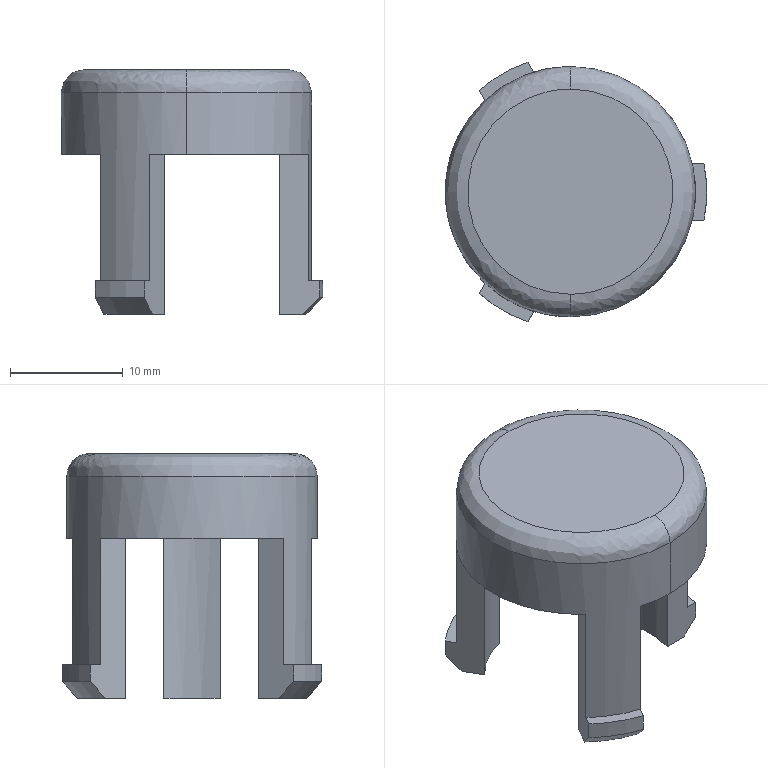Part | SolidWorks | features BaseBody 1 | 1 solid | 30 faces | box 23.2 x 23.006 x 21.7 mm | volume 2251 mm3 | plane 17 | cylinder 7 | cone 4 | spline 2 | commonest cylinder face diameters 24.2 x3 17.2 x2 22.2 x2
STEP:
#1=CARTESIAN_POINT('',(35.731,-11.1,14.8));
#2=VERTEX_POINT('',#1);
#3=CARTESIAN_POINT('',(35.731,11.1,14.8));
#4=VERTEX_POINT('',#3);
#5=CARTESIAN_POINT('',(35.731,0.,14.8));
#6=DIRECTION('',(0.,0.,-1.));
#7=DIRECTION('',(0.,1.,0.));
#8=AXIS2_PLACEMENT_3D('',#5,#6,#7);
#9=CIRCLE('',#8,11.1);
#10=EDGE_CURVE('',#2,#4,#9,.T.);
#11=ORIENTED_EDGE('',*,*,#10,.F.);
#12=CARTESIAN_POINT('',(35.731,-9.1,16.8));
#13=VERTEX_POINT('',#12);
#14=CARTESIAN_POINT('',(35.731,-9.1,14.8));
#15=DIRECTION('',(-1.,0.,0.));
#16=DIRECTION('',(0.,-1.,0.));
#17=AXIS2_PLACEMENT_3D('',#14,#15,#16);
#18=CIRCLE('',#17,2.);
#19=EDGE_CURVE('',#2,#13,#18,.T.);
#20=ORIENTED_EDGE('',*,*,#19,.T.);
#21=CARTESIAN_POINT('',(35.731,9.1,16.8));
#22=VERTEX_POINT('',#21);
#23=CARTESIAN_POINT('',(35.731,-9.1,16.8));
#24=CARTESIAN_POINT('',(17.531,-9.1,16.8));
#25=CARTESIAN_POINT('',(17.531,9.1,16.8));
#26=CARTESIAN_POINT('',(35.731,9.1,16.8));
#27=(BOUNDED_CURVE()B_SPLINE_CURVE(3,(#23,#24,#25,#26),.UNSPECIFIED.,.F.,.T.)B_SPLINE_CURVE_WITH_KNOTS((4,4),(0.,1.),.UNSPECIFIED.)CURVE()GEOMETRIC_REPRESENTATION_ITEM()RATIONAL_B_SPLINE_CURVE((1.,0.3333,0.3333,1.))REPRESENTATION_ITEM(''));
#28=EDGE_CURVE('',#13,#22,#27,.T.);
#29=ORIENTED_EDGE('',*,*,#28,.T.);
#30=CARTESIAN_POINT('',(35.731,9.1,14.8));
#31=DIRECTION('',(1.,0.,0.));
#32=DIRECTION('',(0.,1.,0.));
#33=AXIS2_PLACEMENT_3D('',#30,#31,#32);
#34=CIRCLE('',#33,2.);
#35=EDGE_CURVE('',#4,#22,#34,.T.);
#36=ORIENTED_EDGE('',*,*,#35,.F.);
#37=EDGE_LOOP('',(#11,#20,#29,#36));
#38=FACE_OUTER_BOUND('',#37,.T.);
#39=CARTESIAN_POINT('',(35.731,-11.1,14.8));
#40=CARTESIAN_POINT('',(13.531,-11.1,14.8));
#41=CARTESIAN_POINT('',(13.531,11.1,14.8));
#42=CARTESIAN_POINT('',(35.731,11.1,14.8));
#43=CARTESIAN_POINT('',(35.731,-11.1,15.972));
#44=CARTESIAN_POINT('',(13.531,-11.1,15.972));
#45=CARTESIAN_POINT('',(13.531,11.1,15.972));
#46=CARTESIAN_POINT('',(35.731,11.1,15.972));
#47=CARTESIAN_POINT('',(35.731,-10.272,16.8));
#48=CARTESIAN_POINT('',(15.187,-10.272,16.8));
#49=CARTESIAN_POINT('',(15.187,10.272,16.8));
#50=CARTESIAN_POINT('',(35.731,10.272,16.8));
#51=CARTESIAN_POINT('',(35.731,-9.1,16.8));
#52=CARTESIAN_POINT('',(17.531,-9.1,16.8));
#53=CARTESIAN_POINT('',(17.531,9.1,16.8));
#54=CARTESIAN_POINT('',(35.731,9.1,16.8));
#55=(BOUNDED_SURFACE()B_SPLINE_SURFACE(3,3,((#39,#40,#41,#42),(#43,#44,#45,#46),(#47,#48,#49,#50),(#51,#52,#53,#54)),.UNSPECIFIED.,.F.,.F.,.F.)B_SPLINE_SURFACE_WITH_KNOTS((4,4),(4,4),(0.,1.),(0.,1.),.UNSPECIFIED.)GEOMETRIC_REPRESENTATION_ITEM()RATIONAL_B_SPLINE_SURFACE(((1.,0.3333,0.3333,1.),(0.8047,0.2682,0.2682,0.8047),(0.8047,0.2682,0.2682,0.8047),(1.,0.3333,0.3333,1.)))REPRESENTATION_ITEM('')SURFACE());
#56=ADVANCED_FACE('',(#38),#55,.T.);
#57=CARTESIAN_POINT('',(35.731,0.,14.8));
#58=DIRECTION('',(0.,0.,-1.));
#59=DIRECTION('',(0.,1.,0.));
#60=AXIS2_PLACEMENT_3D('',#57,#58,#59);
#61=CIRCLE('',#60,11.1);
#62=EDGE_CURVE('',#4,#2,#61,.T.);
#63=ORIENTED_EDGE('',*,*,#62,.T.);
#64=CARTESIAN_POINT('',(35.731,-11.1,9.3));
#65=VERTEX_POINT('',#64);
#66=CARTESIAN_POINT('',(35.731,-11.1,53.496));
#67=DIRECTION('',(0.,0.,-1.));
#68=VECTOR('',#67,1000.);
#69=LINE('',#66,#68);
#70=EDGE_CURVE('',#2,#65,#69,.T.);
#71=ORIENTED_EDGE('',*,*,#70,.T.);
#72=CARTESIAN_POINT('',(46.545,-2.5,9.3));
#73=VERTEX_POINT('',#72);
#74=CARTESIAN_POINT('',(35.731,0.,9.3));
#75=DIRECTION('',(0.,0.,1.));
#76=DIRECTION('',(0.,1.,0.));
#77=AXIS2_PLACEMENT_3D('',#74,#75,#76);
#78=CIRCLE('',#77,11.1);
#79=EDGE_CURVE('',#65,#73,#78,.T.);
#80=ORIENTED_EDGE('',*,*,#79,.T.);
#81=CARTESIAN_POINT('',(46.545,-2.5,-1.9));
#82=VERTEX_POINT('',#81);
#83=CARTESIAN_POINT('',(46.545,-2.5,53.496));
#84=DIRECTION('',(0.,0.,-1.));
#85=VECTOR('',#84,1000.);
#86=LINE('',#83,#85);
#87=EDGE_CURVE('',#73,#82,#86,.T.);
#88=ORIENTED_EDGE('',*,*,#87,.T.);
#89=CARTESIAN_POINT('',(46.545,2.5,-1.9));
#90=VERTEX_POINT('',#89);
#91=CARTESIAN_POINT('',(35.731,0.,-1.9));
#92=DIRECTION('',(0.,0.,1.));
#93=DIRECTION('',(0.,1.,0.));
#94=AXIS2_PLACEMENT_3D('',#91,#92,#93);
#95=CIRCLE('',#94,11.1);
#96=EDGE_CURVE('',#82,#90,#95,.T.);
#97=ORIENTED_EDGE('',*,*,#96,.T.);
#98=CARTESIAN_POINT('',(46.545,2.5,9.3));
#99=VERTEX_POINT('',#98);
#100=CARTESIAN_POINT('',(46.545,2.5,53.496));
#101=DIRECTION('',(0.,0.,1.));
#102=VECTOR('',#101,1000.);
#103=LINE('',#100,#102);
#104=EDGE_CURVE('',#90,#99,#103,.T.);
#105=ORIENTED_EDGE('',*,*,#104,.T.);
#106=CARTESIAN_POINT('',(35.731,11.1,9.3));
#107=VERTEX_POINT('',#106);
#108=CARTESIAN_POINT('',(35.731,0.,9.3));
#109=DIRECTION('',(0.,0.,1.));
#110=DIRECTION('',(0.,1.,0.));
#111=AXIS2_PLACEMENT_3D('',#108,#109,#110);
#112=CIRCLE('',#111,11.1);
#113=EDGE_CURVE('',#99,#107,#112,.T.);
#114=ORIENTED_EDGE('',*,*,#113,.T.);
#115=CARTESIAN_POINT('',(35.731,11.1,53.496));
#116=DIRECTION('',(0.,0.,-1.));
#117=VECTOR('',#116,1000.);
#118=LINE('',#115,#117);
#119=EDGE_CURVE('',#4,#107,#118,.T.);
#120=ORIENTED_EDGE('',*,*,#119,.F.);
#121=EDGE_LOOP('',(#63,#71,#80,#88,#97,#105,#114,#120));
#122=FACE_OUTER_BOUND('',#121,.T.);
#123=CARTESIAN_POINT('',(35.731,0.,53.496));
#124=DIRECTION('',(0.,0.,-1.));
#125=DIRECTION('',(0.,1.,0.));
#126=AXIS2_PLACEMENT_3D('',#123,#124,#125);
#127=CYLINDRICAL_SURFACE('',#126,11.1);
#128=ADVANCED_FACE('',(#122),#127,.T.);
#129=CARTESIAN_POINT('',(35.731,-8.6,14.3));
#130=VERTEX_POINT('',#129);
#131=CARTESIAN_POINT('',(35.731,8.6,14.3));
#132=VERTEX_POINT('',#131);
#133=CARTESIAN_POINT('',(35.731,0.,14.3));
#134=DIRECTION('',(0.,0.,-1.));
#135=DIRECTION('',(0.,1.,0.));
#136=AXIS2_PLACEMENT_3D('',#133,#134,#135);
#137=CIRCLE('',#136,8.6);
#138=EDGE_CURVE('',#130,#132,#137,.T.);
#139=ORIENTED_EDGE('',*,*,#138,.F.);
#140=CARTESIAN_POINT('',(35.731,-8.6,9.3));
#141=VERTEX_POINT('',#140);
#142=CARTESIAN_POINT('',(35.731,-8.6,53.496));
#143=DIRECTION('',(0.,0.,-1.));
#144=VECTOR('',#143,1000.);
#145=LINE('',#142,#144);
#146=EDGE_CURVE('',#130,#141,#145,.T.);
#147=ORIENTED_EDGE('',*,*,#146,.T.);
#148=CARTESIAN_POINT('',(33.781,-8.376,9.3));
#149=VERTEX_POINT('',#148);
#150=CARTESIAN_POINT('',(35.731,0.,9.3));
#151=DIRECTION('',(0.,0.,-1.));
#152=DIRECTION('',(0.,1.,0.));
#153=AXIS2_PLACEMENT_3D('',#150,#151,#152);
#154=CIRCLE('',#153,8.6);
#155=EDGE_CURVE('',#141,#149,#154,.T.);
#156=ORIENTED_EDGE('',*,*,#155,.T.);
#157=CARTESIAN_POINT('',(33.781,-8.376,-4.9));
#158=VERTEX_POINT('',#157);
#159=CARTESIAN_POINT('',(33.781,-8.376,-2.4));
#160=DIRECTION('',(0.,0.,-1.));
#161=VECTOR('',#160,1000.);
#162=LINE('',#159,#161);
#163=EDGE_CURVE('',#149,#158,#162,.T.);
#164=ORIENTED_EDGE('',*,*,#163,.T.);
#165=CARTESIAN_POINT('',(29.451,-5.876,-4.9));
#166=VERTEX_POINT('',#165);
#167=CARTESIAN_POINT('',(35.731,0.,-4.9));
#168=DIRECTION('',(0.,0.,1.));
#169=DIRECTION('',(0.,1.,0.));
#170=AXIS2_PLACEMENT_3D('',#167,#168,#169);
#171=CIRCLE('',#170,8.6);
#172=EDGE_CURVE('',#166,#158,#171,.T.);
#173=ORIENTED_EDGE('',*,*,#172,.F.);
#174=CARTESIAN_POINT('',(29.451,-5.876,9.3));
#175=VERTEX_POINT('',#174);
#176=CARTESIAN_POINT('',(29.451,-5.876,-2.4));
#177=DIRECTION('',(0.,0.,1.));
#178=VECTOR('',#177,1000.);
#179=LINE('',#176,#178);
#180=EDGE_CURVE('',#166,#175,#179,.T.);
#181=ORIENTED_EDGE('',*,*,#180,.T.);
#182=CARTESIAN_POINT('',(29.451,5.876,9.3));
#183=VERTEX_POINT('',#182);
#184=CARTESIAN_POINT('',(35.731,0.,9.3));
#185=DIRECTION('',(0.,0.,-1.));
#186=DIRECTION('',(0.,1.,0.));
#187=AXIS2_PLACEMENT_3D('',#184,#185,#186);
#188=CIRCLE('',#187,8.6);
#189=EDGE_CURVE('',#175,#183,#188,.T.);
#190=ORIENTED_EDGE('',*,*,#189,.T.);
#191=CARTESIAN_POINT('',(29.451,5.876,-4.9));
#192=VERTEX_POINT('',#191);
#193=CARTESIAN_POINT('',(29.451,5.876,-1.9));
#194=DIRECTION('',(0.,0.,-1.));
#195=VECTOR('',#194,1000.);
#196=LINE('',#193,#195);
#197=EDGE_CURVE('',#183,#192,#196,.T.);
#198=ORIENTED_EDGE('',*,*,#197,.T.);
#199=CARTESIAN_POINT('',(33.781,8.376,-4.9));
#200=VERTEX_POINT('',#199);
#201=CARTESIAN_POINT('',(35.731,0.,-4.9));
#202=DIRECTION('',(0.,0.,1.));
#203=DIRECTION('',(0.,1.,0.));
#204=AXIS2_PLACEMENT_3D('',#201,#202,#203);
#205=CIRCLE('',#204,8.6);
#206=EDGE_CURVE('',#200,#192,#205,.T.);
#207=ORIENTED_EDGE('',*,*,#206,.F.);
#208=CARTESIAN_POINT('',(33.781,8.376,9.3));
#209=VERTEX_POINT('',#208);
#210=CARTESIAN_POINT('',(33.781,8.376,-1.9));
#211=DIRECTION('',(0.,0.,1.));
#212=VECTOR('',#211,1000.);
#213=LINE('',#210,#212);
#214=EDGE_CURVE('',#200,#209,#213,.T.);
#215=ORIENTED_EDGE('',*,*,#214,.T.);
#216=CARTESIAN_POINT('',(35.731,8.6,9.3));
#217=VERTEX_POINT('',#216);
#218=CARTESIAN_POINT('',(35.731,0.,9.3));
#219=DIRECTION('',(0.,0.,-1.));
#220=DIRECTION('',(0.,1.,0.));
#221=AXIS2_PLACEMENT_3D('',#218,#219,#220);
#222=CIRCLE('',#221,8.6);
#223=EDGE_CURVE('',#209,#217,#222,.T.);
#224=ORIENTED_EDGE('',*,*,#223,.T.);
#225=CARTESIAN_POINT('',(35.731,8.6,53.496));
#226=DIRECTION('',(0.,0.,-1.));
#227=VECTOR('',#226,1000.);
#228=LINE('',#225,#227);
#229=EDGE_CURVE('',#132,#217,#228,.T.);
#230=ORIENTED_EDGE('',*,*,#229,.F.);
#231=EDGE_LOOP('',(#139,#147,#156,#164,#173,#181,#190,#198,#207,#215,#224,#230));
#232=FACE_OUTER_BOUND('',#231,.T.);
#233=CARTESIAN_POINT('',(35.731,0.,53.496));
#234=DIRECTION('',(0.,0.,-1.));
#235=DIRECTION('',(0.,1.,0.));
#236=AXIS2_PLACEMENT_3D('',#233,#234,#235);
#237=CYLINDRICAL_SURFACE('',#236,8.6);
#238=ADVANCED_FACE('',(#232),#237,.F.);
#239=CARTESIAN_POINT('',(46.331,0.,-4.9));
#240=VERTEX_POINT('',#239);
#241=CARTESIAN_POINT('',(46.032,-2.5,-4.9));
#242=VERTEX_POINT('',#241);
#243=CARTESIAN_POINT('',(35.731,0.,-4.9));
#244=DIRECTION('',(0.,0.,-1.));
#245=DIRECTION('',(1.,0.,0.));
#246=AXIS2_PLACEMENT_3D('',#243,#244,#245);
#247=CIRCLE('',#246,10.6);
#248=EDGE_CURVE('',#240,#242,#247,.T.);
#249=ORIENTED_EDGE('',*,*,#248,.F.);
#250=CARTESIAN_POINT('',(47.831,0.,-3.4));
#251=VERTEX_POINT('',#250);
#252=CARTESIAN_POINT('',(47.831,0.,-3.4));
#253=DIRECTION('',(0.7071,0.,0.7071));
#254=VECTOR('',#253,1000.);
#255=LINE('',#252,#254);
#256=EDGE_CURVE('',#240,#251,#255,.T.);
#257=ORIENTED_EDGE('',*,*,#256,.T.);
#258=CARTESIAN_POINT('',(47.569,-2.5,-3.4));
#259=VERTEX_POINT('',#258);
#260=CARTESIAN_POINT('',(35.731,0.,-3.4));
#261=DIRECTION('',(0.,0.,-1.));
#262=DIRECTION('',(1.,0.,0.));
#263=AXIS2_PLACEMENT_3D('',#260,#261,#262);
#264=CIRCLE('',#263,12.1);
#265=EDGE_CURVE('',#251,#259,#264,.T.);
#266=ORIENTED_EDGE('',*,*,#265,.T.);
#267=CARTESIAN_POINT('',(47.569,-2.5,-3.4));
#268=CARTESIAN_POINT('',(47.058,-2.5,-3.901));
#269=CARTESIAN_POINT('',(46.545,-2.5,-4.401));
#270=CARTESIAN_POINT('',(46.032,-2.5,-4.9));
#271=B_SPLINE_CURVE_WITH_KNOTS('',3,(#267,#268,#269,#270),.UNSPECIFIED.,.F.,.F.,(4,4),(0.,0.002148),.UNSPECIFIED.);
#272=EDGE_CURVE('',#259,#242,#271,.T.);
#273=ORIENTED_EDGE('',*,*,#272,.T.);
#274=EDGE_LOOP('',(#249,#257,#266,#273));
#275=FACE_OUTER_BOUND('',#274,.T.);
#276=CARTESIAN_POINT('',(35.731,0.,-3.4));
#277=DIRECTION('',(0.,0.,1.));
#278=DIRECTION('',(1.,0.,0.));
#279=AXIS2_PLACEMENT_3D('',#276,#277,#278);
#280=CONICAL_SURFACE('',#279,12.1,0.7854);
#281=ADVANCED_FACE('',(#275),#280,.T.);
#282=ORIENTED_EDGE('',*,*,#70,.F.);
#283=ORIENTED_EDGE('',*,*,#10,.T.);
#284=ORIENTED_EDGE('',*,*,#119,.T.);
#285=CARTESIAN_POINT('',(32.488,10.616,9.3));
#286=VERTEX_POINT('',#285);
#287=CARTESIAN_POINT('',(35.731,0.,9.3));
#288=DIRECTION('',(0.,0.,1.));
#289=DIRECTION('',(0.,1.,0.));
#290=AXIS2_PLACEMENT_3D('',#287,#288,#289);
#291=CIRCLE('',#290,11.1);
#292=EDGE_CURVE('',#107,#286,#291,.T.);
#293=ORIENTED_EDGE('',*,*,#292,.T.);
#294=CARTESIAN_POINT('',(32.488,10.616,-1.9));
#295=VERTEX_POINT('',#294);
#296=CARTESIAN_POINT('',(32.488,10.616,53.496));
#297=DIRECTION('',(0.,0.,-1.));
#298=VECTOR('',#297,1000.);
#299=LINE('',#296,#298);
#300=EDGE_CURVE('',#286,#295,#299,.T.);
#301=ORIENTED_EDGE('',*,*,#300,.T.);
#302=CARTESIAN_POINT('',(28.158,8.116,-1.9));
#303=VERTEX_POINT('',#302);
#304=CARTESIAN_POINT('',(35.731,0.,-1.9));
#305=DIRECTION('',(0.,0.,1.));
#306=DIRECTION('',(0.,1.,0.));
#307=AXIS2_PLACEMENT_3D('',#304,#305,#306);
#308=CIRCLE('',#307,11.1);
#309=EDGE_CURVE('',#295,#303,#308,.T.);
#310=ORIENTED_EDGE('',*,*,#309,.T.);
#311=CARTESIAN_POINT('',(28.158,8.116,9.3));
#312=VERTEX_POINT('',#311);
#313=CARTESIAN_POINT('',(28.158,8.116,53.496));
#314=DIRECTION('',(0.,0.,1.));
#315=VECTOR('',#314,1000.);
#316=LINE('',#313,#315);
#317=EDGE_CURVE('',#303,#312,#316,.T.);
#318=ORIENTED_EDGE('',*,*,#317,.T.);
#319=CARTESIAN_POINT('',(28.158,-8.116,9.3));
#320=VERTEX_POINT('',#319);
#321=CARTESIAN_POINT('',(35.731,0.,9.3));
#322=DIRECTION('',(0.,0.,1.));
#323=DIRECTION('',(0.,1.,0.));
#324=AXIS2_PLACEMENT_3D('',#321,#322,#323);
#325=CIRCLE('',#324,11.1);
#326=EDGE_CURVE('',#312,#320,#325,.T.);
#327=ORIENTED_EDGE('',*,*,#326,.T.);
#328=CARTESIAN_POINT('',(28.158,-8.116,-1.9));
#329=VERTEX_POINT('',#328);
#330=CARTESIAN_POINT('',(28.158,-8.116,53.496));
#331=DIRECTION('',(0.,0.,-1.));
#332=VECTOR('',#331,1000.);
#333=LINE('',#330,#332);
#334=EDGE_CURVE('',#320,#329,#333,.T.);
#335=ORIENTED_EDGE('',*,*,#334,.T.);
#336=CARTESIAN_POINT('',(32.488,-10.616,-1.9));
#337=VERTEX_POINT('',#336);
#338=CARTESIAN_POINT('',(35.731,0.,-1.9));
#339=DIRECTION('',(0.,0.,1.));
#340=DIRECTION('',(0.,1.,0.));
#341=AXIS2_PLACEMENT_3D('',#338,#339,#340);
#342=CIRCLE('',#341,11.1);
#343=EDGE_CURVE('',#329,#337,#342,.T.);
#344=ORIENTED_EDGE('',*,*,#343,.T.);
#345=CARTESIAN_POINT('',(32.488,-10.616,9.3));
#346=VERTEX_POINT('',#345);
#347=CARTESIAN_POINT('',(32.488,-10.616,53.496));
#348=DIRECTION('',(0.,0.,1.));
#349=VECTOR('',#348,1000.);
#350=LINE('',#347,#349);
#351=EDGE_CURVE('',#337,#346,#350,.T.);
#352=ORIENTED_EDGE('',*,*,#351,.T.);
#353=CARTESIAN_POINT('',(35.731,0.,9.3));
#354=DIRECTION('',(0.,0.,1.));
#355=DIRECTION('',(0.,1.,0.));
#356=AXIS2_PLACEMENT_3D('',#353,#354,#355);
#357=CIRCLE('',#356,11.1);
#358=EDGE_CURVE('',#346,#65,#357,.T.);
#359=ORIENTED_EDGE('',*,*,#358,.T.);
#360=EDGE_LOOP('',(#282,#283,#284,#293,#301,#310,#318,#327,#335,#344,#352,#359));
#361=FACE_OUTER_BOUND('',#360,.T.);
#362=CARTESIAN_POINT('',(35.731,0.,53.496));
#363=DIRECTION('',(0.,0.,-1.));
#364=DIRECTION('',(0.,1.,0.));
#365=AXIS2_PLACEMENT_3D('',#362,#363,#364);
#366=CYLINDRICAL_SURFACE('',#365,11.1);
#367=ADVANCED_FACE('',(#361),#366,.T.);
#368=CARTESIAN_POINT('',(43.959,-2.5,9.3));
#369=VERTEX_POINT('',#368);
#370=CARTESIAN_POINT('',(55.234,-2.5,9.3));
#371=DIRECTION('',(-1.,0.,0.));
#372=VECTOR('',#371,1000.);
#373=LINE('',#370,#372);
#374=EDGE_CURVE('',#73,#369,#373,.T.);
#375=ORIENTED_EDGE('',*,*,#374,.F.);
#376=ORIENTED_EDGE('',*,*,#79,.F.);
#377=ORIENTED_EDGE('',*,*,#358,.F.);
#378=CARTESIAN_POINT('',(33.781,-8.376,9.3));
#379=DIRECTION('',(-0.5,-0.866,0.));
#380=VECTOR('',#379,1000.);
#381=LINE('',#378,#380);
#382=EDGE_CURVE('',#149,#346,#381,.T.);
#383=ORIENTED_EDGE('',*,*,#382,.F.);
#384=ORIENTED_EDGE('',*,*,#155,.F.);
#385=CARTESIAN_POINT('',(35.731,0.,9.3));
#386=DIRECTION('',(0.,0.,-1.));
#387=DIRECTION('',(0.,1.,0.));
#388=AXIS2_PLACEMENT_3D('',#385,#386,#387);
#389=CIRCLE('',#388,8.6);
#390=EDGE_CURVE('',#369,#141,#389,.T.);
#391=ORIENTED_EDGE('',*,*,#390,.F.);
#392=EDGE_LOOP('',(#375,#376,#377,#383,#384,#391));
#393=FACE_OUTER_BOUND('',#392,.T.);
#394=CARTESIAN_POINT('',(55.234,1.301,9.3));
#395=DIRECTION('',(0.,0.,1.));
#396=DIRECTION('',(0.,-1.,0.));
#397=AXIS2_PLACEMENT_3D('',#394,#395,#396);
#398=PLANE('',#397);
#399=ADVANCED_FACE('',(#393),#398,.F.);
#400=CARTESIAN_POINT('',(31.976,-11.503,-3.4));
#401=VERTEX_POINT('',#400);
#402=CARTESIAN_POINT('',(31.976,-11.503,-1.9));
#403=VERTEX_POINT('',#402);
#404=CARTESIAN_POINT('',(31.976,-11.503,-4.9));
#405=DIRECTION('',(0.,0.,1.));
#406=VECTOR('',#405,1000.);
#407=LINE('',#404,#406);
#408=EDGE_CURVE('',#401,#403,#407,.T.);
#409=ORIENTED_EDGE('',*,*,#408,.F.);
#410=CARTESIAN_POINT('',(32.745,-10.171,-4.9));
#411=VERTEX_POINT('',#410);
#412=CARTESIAN_POINT('',(32.745,-10.171,-4.9));
#413=CARTESIAN_POINT('',(32.488,-10.616,-4.401));
#414=CARTESIAN_POINT('',(32.232,-11.06,-3.901));
#415=CARTESIAN_POINT('',(31.976,-11.503,-3.4));
#416=B_SPLINE_CURVE_WITH_KNOTS('',3,(#412,#413,#414,#415),.UNSPECIFIED.,.F.,.F.,(4,4),(0.,0.002148),.UNSPECIFIED.);
#417=EDGE_CURVE('',#411,#401,#416,.T.);
#418=ORIENTED_EDGE('',*,*,#417,.F.);
#419=CARTESIAN_POINT('',(33.781,-8.376,-4.9));
#420=DIRECTION('',(-0.5,-0.866,0.));
#421=VECTOR('',#420,1000.);
#422=LINE('',#419,#421);
#423=EDGE_CURVE('',#158,#411,#422,.T.);
#424=ORIENTED_EDGE('',*,*,#423,.F.);
#425=ORIENTED_EDGE('',*,*,#163,.F.);
#426=ORIENTED_EDGE('',*,*,#382,.T.);
#427=ORIENTED_EDGE('',*,*,#351,.F.);
#428=CARTESIAN_POINT('',(33.781,-8.376,-1.9));
#429=DIRECTION('',(0.5,0.866,0.));
#430=VECTOR('',#429,1000.);
#431=LINE('',#428,#430);
#432=EDGE_CURVE('',#403,#337,#431,.T.);
#433=ORIENTED_EDGE('',*,*,#432,.F.);
#434=EDGE_LOOP('',(#409,#418,#424,#425,#426,#427,#433));
#435=FACE_OUTER_BOUND('',#434,.T.);
#436=CARTESIAN_POINT('',(33.781,-8.376,-2.4));
#437=DIRECTION('',(-0.866,0.5,0.));
#438=DIRECTION('',(-0.5,-0.866,0.));
#439=AXIS2_PLACEMENT_3D('',#436,#437,#438);
#440=PLANE('',#439);
#441=ADVANCED_FACE('',(#435),#440,.F.);
#442=CARTESIAN_POINT('',(27.646,-9.003,-1.9));
#443=VERTEX_POINT('',#442);
#444=CARTESIAN_POINT('',(35.731,0.,-1.9));
#445=DIRECTION('',(0.,0.,-1.));
#446=DIRECTION('',(0.,-1.,0.));
#447=AXIS2_PLACEMENT_3D('',#444,#445,#446);
#448=CIRCLE('',#447,12.1);
#449=EDGE_CURVE('',#403,#443,#448,.T.);
#450=ORIENTED_EDGE('',*,*,#449,.F.);
#451=ORIENTED_EDGE('',*,*,#432,.T.);
#452=ORIENTED_EDGE('',*,*,#343,.F.);
#453=CARTESIAN_POINT('',(27.646,-9.003,-1.9));
#454=DIRECTION('',(0.5,0.866,0.));
#455=VECTOR('',#454,1000.);
#456=LINE('',#453,#455);
#457=EDGE_CURVE('',#443,#329,#456,.T.);
#458=ORIENTED_EDGE('',*,*,#457,.F.);
#459=EDGE_LOOP('',(#450,#451,#452,#458));
#460=FACE_OUTER_BOUND('',#459,.T.);
#461=CARTESIAN_POINT('',(35.731,0.,-1.9));
#462=DIRECTION('',(0.,0.,-1.));
#463=DIRECTION('',(0.,1.,0.));
#464=AXIS2_PLACEMENT_3D('',#461,#462,#463);
#465=PLANE('',#464);
#466=ADVANCED_FACE('',(#460),#465,.F.);
#467=CARTESIAN_POINT('',(27.646,-9.003,-3.4));
#468=VERTEX_POINT('',#467);
#469=CARTESIAN_POINT('',(28.415,-7.671,-4.9));
#470=VERTEX_POINT('',#469);
#471=CARTESIAN_POINT('',(27.646,-9.003,-3.4));
#472=CARTESIAN_POINT('',(27.902,-8.56,-3.901));
#473=CARTESIAN_POINT('',(28.158,-8.116,-4.401));
#474=CARTESIAN_POINT('',(28.415,-7.671,-4.9));
#475=B_SPLINE_CURVE_WITH_KNOTS('',3,(#471,#472,#473,#474),.UNSPECIFIED.,.F.,.F.,(4,4),(0.,0.002148),.UNSPECIFIED.);
#476=EDGE_CURVE('',#468,#470,#475,.T.);
#477=ORIENTED_EDGE('',*,*,#476,.F.);
#478=CARTESIAN_POINT('',(27.646,-9.003,-2.4));
#479=DIRECTION('',(0.,0.,-1.));
#480=VECTOR('',#479,1000.);
#481=LINE('',#478,#480);
#482=EDGE_CURVE('',#443,#468,#481,.T.);
#483=ORIENTED_EDGE('',*,*,#482,.F.);
#484=ORIENTED_EDGE('',*,*,#457,.T.);
#485=ORIENTED_EDGE('',*,*,#334,.F.);
#486=CARTESIAN_POINT('',(28.158,-8.116,9.3));
#487=DIRECTION('',(-0.5,-0.866,0.));
#488=VECTOR('',#487,1000.);
#489=LINE('',#486,#488);
#490=EDGE_CURVE('',#175,#320,#489,.T.);
#491=ORIENTED_EDGE('',*,*,#490,.F.);
#492=ORIENTED_EDGE('',*,*,#180,.F.);
#493=CARTESIAN_POINT('',(28.158,-8.116,-4.9));
#494=DIRECTION('',(0.5,0.866,0.));
#495=VECTOR('',#494,1000.);
#496=LINE('',#493,#495);
#497=EDGE_CURVE('',#470,#166,#496,.T.);
#498=ORIENTED_EDGE('',*,*,#497,.F.);
#499=EDGE_LOOP('',(#477,#483,#484,#485,#491,#492,#498));
#500=FACE_OUTER_BOUND('',#499,.T.);
#501=CARTESIAN_POINT('',(28.158,-8.116,-2.4));
#502=DIRECTION('',(0.866,-0.5,0.));
#503=DIRECTION('',(0.5,0.866,0.));
#504=AXIS2_PLACEMENT_3D('',#501,#502,#503);
#505=PLANE('',#504);
#506=ADVANCED_FACE('',(#500),#505,.F.);
#507=CARTESIAN_POINT('',(29.451,5.876,9.3));
#508=DIRECTION('',(-0.5,0.866,0.));
#509=VECTOR('',#508,1000.);
#510=LINE('',#507,#509);
#511=EDGE_CURVE('',#183,#312,#510,.T.);
#512=ORIENTED_EDGE('',*,*,#511,.F.);
#513=ORIENTED_EDGE('',*,*,#189,.F.);
#514=ORIENTED_EDGE('',*,*,#490,.T.);
#515=ORIENTED_EDGE('',*,*,#326,.F.);
#516=EDGE_LOOP('',(#512,#513,#514,#515));
#517=FACE_OUTER_BOUND('',#516,.T.);
#518=CARTESIAN_POINT('',(55.234,1.301,9.3));
#519=DIRECTION('',(0.,0.,1.));
#520=DIRECTION('',(0.,-1.,0.));
#521=AXIS2_PLACEMENT_3D('',#518,#519,#520);
#522=PLANE('',#521);
#523=ADVANCED_FACE('',(#517),#522,.F.);
#524=CARTESIAN_POINT('',(27.646,9.003,-3.4));
#525=VERTEX_POINT('',#524);
#526=CARTESIAN_POINT('',(27.646,9.003,-1.9));
#527=VERTEX_POINT('',#526);
#528=CARTESIAN_POINT('',(27.646,9.003,-4.9));
#529=DIRECTION('',(0.,0.,1.));
#530=VECTOR('',#529,1000.);
#531=LINE('',#528,#530);
#532=EDGE_CURVE('',#525,#527,#531,.T.);
#533=ORIENTED_EDGE('',*,*,#532,.F.);
#534=CARTESIAN_POINT('',(28.415,7.671,-4.9));
#535=VERTEX_POINT('',#534);
#536=CARTESIAN_POINT('',(28.415,7.671,-4.9));
#537=CARTESIAN_POINT('',(28.158,8.116,-4.401));
#538=CARTESIAN_POINT('',(27.902,8.56,-3.901));
#539=CARTESIAN_POINT('',(27.646,9.003,-3.4));
#540=B_SPLINE_CURVE_WITH_KNOTS('',3,(#536,#537,#538,#539),.UNSPECIFIED.,.F.,.F.,(4,4),(0.,0.002148),.UNSPECIFIED.);
#541=EDGE_CURVE('',#535,#525,#540,.T.);
#542=ORIENTED_EDGE('',*,*,#541,.F.);
#543=CARTESIAN_POINT('',(29.451,5.876,-4.9));
#544=DIRECTION('',(-0.5,0.866,0.));
#545=VECTOR('',#544,1000.);
#546=LINE('',#543,#545);
#547=EDGE_CURVE('',#192,#535,#546,.T.);
#548=ORIENTED_EDGE('',*,*,#547,.F.);
#549=ORIENTED_EDGE('',*,*,#197,.F.);
#550=ORIENTED_EDGE('',*,*,#511,.T.);
#551=ORIENTED_EDGE('',*,*,#317,.F.);
#552=CARTESIAN_POINT('',(29.451,5.876,-1.9));
#553=DIRECTION('',(0.5,-0.866,0.));
#554=VECTOR('',#553,1000.);
#555=LINE('',#552,#554);
#556=EDGE_CURVE('',#527,#303,#555,.T.);
#557=ORIENTED_EDGE('',*,*,#556,.F.);
#558=EDGE_LOOP('',(#533,#542,#548,#549,#550,#551,#557));
#559=FACE_OUTER_BOUND('',#558,.T.);
#560=CARTESIAN_POINT('',(29.451,5.876,-1.9));
#561=DIRECTION('',(0.866,0.5,0.));
#562=DIRECTION('',(-0.5,0.866,0.));
#563=AXIS2_PLACEMENT_3D('',#560,#561,#562);
#564=PLANE('',#563);
#565=ADVANCED_FACE('',(#559),#564,.F.);
#566=CARTESIAN_POINT('',(31.976,11.503,-1.9));
#567=VERTEX_POINT('',#566);
#568=CARTESIAN_POINT('',(35.731,0.,-1.9));
#569=DIRECTION('',(0.,0.,-1.));
#570=DIRECTION('',(0.,-1.,0.));
#571=AXIS2_PLACEMENT_3D('',#568,#569,#570);
#572=CIRCLE('',#571,12.1);
#573=EDGE_CURVE('',#527,#567,#572,.T.);
#574=ORIENTED_EDGE('',*,*,#573,.F.);
#575=ORIENTED_EDGE('',*,*,#556,.T.);
#576=ORIENTED_EDGE('',*,*,#309,.F.);
#577=CARTESIAN_POINT('',(31.976,11.503,-1.9));
#578=DIRECTION('',(0.5,-0.866,0.));
#579=VECTOR('',#578,1000.);
#580=LINE('',#577,#579);
#581=EDGE_CURVE('',#567,#295,#580,.T.);
#582=ORIENTED_EDGE('',*,*,#581,.F.);
#583=EDGE_LOOP('',(#574,#575,#576,#582));
#584=FACE_OUTER_BOUND('',#583,.T.);
#585=CARTESIAN_POINT('',(35.731,0.,-1.9));
#586=DIRECTION('',(0.,0.,-1.));
#587=DIRECTION('',(0.,1.,0.));
#588=AXIS2_PLACEMENT_3D('',#585,#586,#587);
#589=PLANE('',#588);
#590=ADVANCED_FACE('',(#584),#589,.F.);
#591=CARTESIAN_POINT('',(31.976,11.503,-3.4));
#592=VERTEX_POINT('',#591);
#593=CARTESIAN_POINT('',(32.745,10.171,-4.9));
#594=VERTEX_POINT('',#593);
#595=CARTESIAN_POINT('',(31.976,11.503,-3.4));
#596=CARTESIAN_POINT('',(32.232,11.06,-3.901));
#597=CARTESIAN_POINT('',(32.488,10.616,-4.401));
#598=CARTESIAN_POINT('',(32.745,10.171,-4.9));
#599=B_SPLINE_CURVE_WITH_KNOTS('',3,(#595,#596,#597,#598),.UNSPECIFIED.,.F.,.F.,(4,4),(0.,0.002148),.UNSPECIFIED.);
#600=EDGE_CURVE('',#592,#594,#599,.T.);
#601=ORIENTED_EDGE('',*,*,#600,.F.);
#602=CARTESIAN_POINT('',(31.976,11.503,-1.9));
#603=DIRECTION('',(0.,0.,-1.));
#604=VECTOR('',#603,1000.);
#605=LINE('',#602,#604);
#606=EDGE_CURVE('',#567,#592,#605,.T.);
#607=ORIENTED_EDGE('',*,*,#606,.F.);
#608=ORIENTED_EDGE('',*,*,#581,.T.);
#609=ORIENTED_EDGE('',*,*,#300,.F.);
#610=CARTESIAN_POINT('',(32.488,10.616,9.3));
#611=DIRECTION('',(-0.5,0.866,0.));
#612=VECTOR('',#611,1000.);
#613=LINE('',#610,#612);
#614=EDGE_CURVE('',#209,#286,#613,.T.);
#615=ORIENTED_EDGE('',*,*,#614,.F.);
#616=ORIENTED_EDGE('',*,*,#214,.F.);
#617=CARTESIAN_POINT('',(32.488,10.616,-4.9));
#618=DIRECTION('',(0.5,-0.866,0.));
#619=VECTOR('',#618,1000.);
#620=LINE('',#617,#619);
#621=EDGE_CURVE('',#594,#200,#620,.T.);
#622=ORIENTED_EDGE('',*,*,#621,.F.);
#623=EDGE_LOOP('',(#601,#607,#608,#609,#615,#616,#622));
#624=FACE_OUTER_BOUND('',#623,.T.);
#625=CARTESIAN_POINT('',(32.488,10.616,-1.9));
#626=DIRECTION('',(-0.866,-0.5,0.));
#627=DIRECTION('',(0.5,-0.866,0.));
#628=AXIS2_PLACEMENT_3D('',#625,#626,#627);
#629=PLANE('',#628);
#630=ADVANCED_FACE('',(#624),#629,.F.);
#631=ORIENTED_EDGE('',*,*,#614,.T.);
#632=ORIENTED_EDGE('',*,*,#292,.F.);
#633=ORIENTED_EDGE('',*,*,#113,.F.);
#634=CARTESIAN_POINT('',(43.959,2.5,9.3));
#635=VERTEX_POINT('',#634);
#636=CARTESIAN_POINT('',(55.234,2.5,9.3));
#637=DIRECTION('',(1.,0.,0.));
#638=VECTOR('',#637,1000.);
#639=LINE('',#636,#638);
#640=EDGE_CURVE('',#635,#99,#639,.T.);
#641=ORIENTED_EDGE('',*,*,#640,.F.);
#642=CARTESIAN_POINT('',(35.731,0.,9.3));
#643=DIRECTION('',(0.,0.,-1.));
#644=DIRECTION('',(0.,1.,0.));
#645=AXIS2_PLACEMENT_3D('',#642,#643,#644);
#646=CIRCLE('',#645,8.6);
#647=EDGE_CURVE('',#217,#635,#646,.T.);
#648=ORIENTED_EDGE('',*,*,#647,.F.);
#649=ORIENTED_EDGE('',*,*,#223,.F.);
#650=EDGE_LOOP('',(#631,#632,#633,#641,#648,#649));
#651=FACE_OUTER_BOUND('',#650,.T.);
#652=CARTESIAN_POINT('',(55.234,1.301,9.3));
#653=DIRECTION('',(0.,0.,1.));
#654=DIRECTION('',(0.,-1.,0.));
#655=AXIS2_PLACEMENT_3D('',#652,#653,#654);
#656=PLANE('',#655);
#657=ADVANCED_FACE('',(#651),#656,.F.);
#658=ORIENTED_EDGE('',*,*,#19,.F.);
#659=ORIENTED_EDGE('',*,*,#62,.F.);
#660=ORIENTED_EDGE('',*,*,#35,.T.);
#661=CARTESIAN_POINT('',(35.731,9.1,16.8));
#662=CARTESIAN_POINT('',(53.931,9.1,16.8));
#663=CARTESIAN_POINT('',(53.931,-9.1,16.8));
#664=CARTESIAN_POINT('',(35.731,-9.1,16.8));
#665=(BOUNDED_CURVE()B_SPLINE_CURVE(3,(#661,#662,#663,#664),.UNSPECIFIED.,.F.,.T.)B_SPLINE_CURVE_WITH_KNOTS((4,4),(0.,1.),.UNSPECIFIED.)CURVE()GEOMETRIC_REPRESENTATION_ITEM()RATIONAL_B_SPLINE_CURVE((1.,0.3333,0.3333,1.))REPRESENTATION_ITEM(''));
#666=EDGE_CURVE('',#22,#13,#665,.T.);
#667=ORIENTED_EDGE('',*,*,#666,.T.);
#668=EDGE_LOOP('',(#658,#659,#660,#667));
#669=FACE_OUTER_BOUND('',#668,.T.);
#670=CARTESIAN_POINT('',(35.731,11.1,14.8));
#671=CARTESIAN_POINT('',(57.931,11.1,14.8));
#672=CARTESIAN_POINT('',(57.931,-11.1,14.8));
#673=CARTESIAN_POINT('',(35.731,-11.1,14.8));
#674=CARTESIAN_POINT('',(35.731,11.1,15.972));
#675=CARTESIAN_POINT('',(57.931,11.1,15.972));
#676=CARTESIAN_POINT('',(57.931,-11.1,15.972));
#677=CARTESIAN_POINT('',(35.731,-11.1,15.972));
#678=CARTESIAN_POINT('',(35.731,10.272,16.8));
#679=CARTESIAN_POINT('',(56.274,10.272,16.8));
#680=CARTESIAN_POINT('',(56.274,-10.272,16.8));
#681=CARTESIAN_POINT('',(35.731,-10.272,16.8));
#682=CARTESIAN_POINT('',(35.731,9.1,16.8));
#683=CARTESIAN_POINT('',(53.931,9.1,16.8));
#684=CARTESIAN_POINT('',(53.931,-9.1,16.8));
#685=CARTESIAN_POINT('',(35.731,-9.1,16.8));
#686=(BOUNDED_SURFACE()B_SPLINE_SURFACE(3,3,((#670,#671,#672,#673),(#674,#675,#676,#677),(#678,#679,#680,#681),(#682,#683,#684,#685)),.UNSPECIFIED.,.F.,.F.,.T.)B_SPLINE_SURFACE_WITH_KNOTS((4,4),(4,4),(0.,1.),(0.,1.),.UNSPECIFIED.)GEOMETRIC_REPRESENTATION_ITEM()RATIONAL_B_SPLINE_SURFACE(((1.,0.3333,0.3333,1.),(0.8047,0.2682,0.2682,0.8047),(0.8047,0.2682,0.2682,0.8047),(1.,0.3333,0.3333,1.)))REPRESENTATION_ITEM('')SURFACE());
#687=ADVANCED_FACE('',(#669),#686,.T.);
#688=ORIENTED_EDGE('',*,*,#272,.F.);
#689=CARTESIAN_POINT('',(47.569,-2.5,-1.9));
#690=VERTEX_POINT('',#689);
#691=CARTESIAN_POINT('',(47.569,-2.5,-4.9));
#692=DIRECTION('',(0.,0.,-1.));
#693=VECTOR('',#692,1000.);
#694=LINE('',#691,#693);
#695=EDGE_CURVE('',#690,#259,#694,.T.);
#696=ORIENTED_EDGE('',*,*,#695,.F.);
#697=CARTESIAN_POINT('',(46.545,-2.5,-1.9));
#698=DIRECTION('',(1.,0.,0.));
#699=VECTOR('',#698,1000.);
#700=LINE('',#697,#699);
#701=EDGE_CURVE('',#82,#690,#700,.T.);
#702=ORIENTED_EDGE('',*,*,#701,.F.);
#703=ORIENTED_EDGE('',*,*,#87,.F.);
#704=ORIENTED_EDGE('',*,*,#374,.T.);
#705=CARTESIAN_POINT('',(43.959,-2.5,-4.9));
#706=VERTEX_POINT('',#705);
#707=CARTESIAN_POINT('',(43.959,-2.5,-2.4));
#708=DIRECTION('',(0.,0.,1.));
#709=VECTOR('',#708,1000.);
#710=LINE('',#707,#709);
#711=EDGE_CURVE('',#706,#369,#710,.T.);
#712=ORIENTED_EDGE('',*,*,#711,.F.);
#713=CARTESIAN_POINT('',(46.545,-2.5,-4.9));
#714=DIRECTION('',(-1.,0.,0.));
#715=VECTOR('',#714,1000.);
#716=LINE('',#713,#715);
#717=EDGE_CURVE('',#242,#706,#716,.T.);
#718=ORIENTED_EDGE('',*,*,#717,.F.);
#719=EDGE_LOOP('',(#688,#696,#702,#703,#704,#712,#718));
#720=FACE_OUTER_BOUND('',#719,.T.);
#721=CARTESIAN_POINT('',(46.545,-2.5,-2.4));
#722=DIRECTION('',(0.,1.,0.));
#723=DIRECTION('',(0.,0.,1.));
#724=AXIS2_PLACEMENT_3D('',#721,#722,#723);
#725=PLANE('',#724);
#726=ADVANCED_FACE('',(#720),#725,.F.);
#727=ORIENTED_EDGE('',*,*,#146,.F.);
#728=CARTESIAN_POINT('',(35.731,0.,14.3));
#729=DIRECTION('',(0.,0.,-1.));
#730=DIRECTION('',(0.,1.,0.));
#731=AXIS2_PLACEMENT_3D('',#728,#729,#730);
#732=CIRCLE('',#731,8.6);
#733=EDGE_CURVE('',#132,#130,#732,.T.);
#734=ORIENTED_EDGE('',*,*,#733,.F.);
#735=ORIENTED_EDGE('',*,*,#229,.T.);
#736=ORIENTED_EDGE('',*,*,#647,.T.);
#737=CARTESIAN_POINT('',(43.959,2.5,-4.9));
#738=VERTEX_POINT('',#737);
#739=CARTESIAN_POINT('',(43.959,2.5,53.496));
#740=DIRECTION('',(0.,0.,1.));
#741=VECTOR('',#740,1000.);
#742=LINE('',#739,#741);
#743=EDGE_CURVE('',#738,#635,#742,.T.);
#744=ORIENTED_EDGE('',*,*,#743,.F.);
#745=CARTESIAN_POINT('',(35.731,0.,-4.9));
#746=DIRECTION('',(0.,0.,1.));
#747=DIRECTION('',(0.,1.,0.));
#748=AXIS2_PLACEMENT_3D('',#745,#746,#747);
#749=CIRCLE('',#748,8.6);
#750=EDGE_CURVE('',#706,#738,#749,.T.);
#751=ORIENTED_EDGE('',*,*,#750,.F.);
#752=ORIENTED_EDGE('',*,*,#711,.T.);
#753=ORIENTED_EDGE('',*,*,#390,.T.);
#754=EDGE_LOOP('',(#727,#734,#735,#736,#744,#751,#752,#753));
#755=FACE_OUTER_BOUND('',#754,.T.);
#756=CARTESIAN_POINT('',(35.731,0.,53.496));
#757=DIRECTION('',(0.,0.,-1.));
#758=DIRECTION('',(0.,1.,0.));
#759=AXIS2_PLACEMENT_3D('',#756,#757,#758);
#760=CYLINDRICAL_SURFACE('',#759,8.6);
#761=ADVANCED_FACE('',(#755),#760,.F.);
#762=ORIENTED_EDGE('',*,*,#476,.T.);
#763=CARTESIAN_POINT('',(35.731,0.,-4.9));
#764=DIRECTION('',(0.,0.,1.));
#765=DIRECTION('',(0.,-1.,0.));
#766=AXIS2_PLACEMENT_3D('',#763,#764,#765);
#767=CIRCLE('',#766,10.6);
#768=EDGE_CURVE('',#470,#411,#767,.T.);
#769=ORIENTED_EDGE('',*,*,#768,.T.);
#770=ORIENTED_EDGE('',*,*,#417,.T.);
#771=CARTESIAN_POINT('',(35.731,0.,-3.4));
#772=DIRECTION('',(0.,0.,-1.));
#773=DIRECTION('',(0.,-1.,0.));
#774=AXIS2_PLACEMENT_3D('',#771,#772,#773);
#775=CIRCLE('',#774,12.1);
#776=EDGE_CURVE('',#401,#468,#775,.T.);
#777=ORIENTED_EDGE('',*,*,#776,.T.);
#778=EDGE_LOOP('',(#762,#769,#770,#777));
#779=FACE_OUTER_BOUND('',#778,.T.);
#780=CARTESIAN_POINT('',(35.731,0.,-3.4));
#781=DIRECTION('',(0.,0.,1.));
#782=DIRECTION('',(0.,-1.,0.));
#783=AXIS2_PLACEMENT_3D('',#780,#781,#782);
#784=CONICAL_SURFACE('',#783,12.1,0.7854);
#785=ADVANCED_FACE('',(#779),#784,.T.);
#786=ORIENTED_EDGE('',*,*,#497,.T.);
#787=ORIENTED_EDGE('',*,*,#172,.T.);
#788=ORIENTED_EDGE('',*,*,#423,.T.);
#789=ORIENTED_EDGE('',*,*,#768,.F.);
#790=EDGE_LOOP('',(#786,#787,#788,#789));
#791=FACE_OUTER_BOUND('',#790,.T.);
#792=CARTESIAN_POINT('',(35.731,0.,-4.9));
#793=DIRECTION('',(0.,0.,-1.));
#794=DIRECTION('',(0.,1.,0.));
#795=AXIS2_PLACEMENT_3D('',#792,#793,#794);
#796=PLANE('',#795);
#797=ADVANCED_FACE('',(#791),#796,.T.);
#798=ORIENTED_EDGE('',*,*,#408,.T.);
#799=ORIENTED_EDGE('',*,*,#449,.T.);
#800=ORIENTED_EDGE('',*,*,#482,.T.);
#801=ORIENTED_EDGE('',*,*,#776,.F.);
#802=EDGE_LOOP('',(#798,#799,#800,#801));
#803=FACE_OUTER_BOUND('',#802,.T.);
#804=CARTESIAN_POINT('',(35.731,0.,-4.9));
#805=DIRECTION('',(0.,0.,1.));
#806=DIRECTION('',(0.,-1.,0.));
#807=AXIS2_PLACEMENT_3D('',#804,#805,#806);
#808=CYLINDRICAL_SURFACE('',#807,12.1);
#809=ADVANCED_FACE('',(#803),#808,.T.);
#810=ORIENTED_EDGE('',*,*,#600,.T.);
#811=CARTESIAN_POINT('',(35.731,0.,-4.9));
#812=DIRECTION('',(0.,0.,1.));
#813=DIRECTION('',(0.,-1.,0.));
#814=AXIS2_PLACEMENT_3D('',#811,#812,#813);
#815=CIRCLE('',#814,10.6);
#816=EDGE_CURVE('',#594,#535,#815,.T.);
#817=ORIENTED_EDGE('',*,*,#816,.T.);
#818=ORIENTED_EDGE('',*,*,#541,.T.);
#819=CARTESIAN_POINT('',(35.731,0.,-3.4));
#820=DIRECTION('',(0.,0.,-1.));
#821=DIRECTION('',(0.,-1.,0.));
#822=AXIS2_PLACEMENT_3D('',#819,#820,#821);
#823=CIRCLE('',#822,12.1);
#824=EDGE_CURVE('',#525,#592,#823,.T.);
#825=ORIENTED_EDGE('',*,*,#824,.T.);
#826=EDGE_LOOP('',(#810,#817,#818,#825));
#827=FACE_OUTER_BOUND('',#826,.T.);
#828=CARTESIAN_POINT('',(35.731,0.,-3.4));
#829=DIRECTION('',(0.,0.,1.));
#830=DIRECTION('',(0.,-1.,0.));
#831=AXIS2_PLACEMENT_3D('',#828,#829,#830);
#832=CONICAL_SURFACE('',#831,12.1,0.7854);
#833=ADVANCED_FACE('',(#827),#832,.T.);
#834=ORIENTED_EDGE('',*,*,#621,.T.);
#835=ORIENTED_EDGE('',*,*,#206,.T.);
#836=ORIENTED_EDGE('',*,*,#547,.T.);
#837=ORIENTED_EDGE('',*,*,#816,.F.);
#838=EDGE_LOOP('',(#834,#835,#836,#837));
#839=FACE_OUTER_BOUND('',#838,.T.);
#840=CARTESIAN_POINT('',(35.731,0.,-4.9));
#841=DIRECTION('',(0.,0.,-1.));
#842=DIRECTION('',(0.,1.,0.));
#843=AXIS2_PLACEMENT_3D('',#840,#841,#842);
#844=PLANE('',#843);
#845=ADVANCED_FACE('',(#839),#844,.T.);
#846=ORIENTED_EDGE('',*,*,#532,.T.);
#847=ORIENTED_EDGE('',*,*,#573,.T.);
#848=ORIENTED_EDGE('',*,*,#606,.T.);
#849=ORIENTED_EDGE('',*,*,#824,.F.);
#850=EDGE_LOOP('',(#846,#847,#848,#849));
#851=FACE_OUTER_BOUND('',#850,.T.);
#852=CARTESIAN_POINT('',(35.731,0.,-4.9));
#853=DIRECTION('',(0.,0.,1.));
#854=DIRECTION('',(0.,-1.,0.));
#855=AXIS2_PLACEMENT_3D('',#852,#853,#854);
#856=CYLINDRICAL_SURFACE('',#855,12.1);
#857=ADVANCED_FACE('',(#851),#856,.T.);
#858=CARTESIAN_POINT('',(47.569,2.5,-3.4));
#859=VERTEX_POINT('',#858);
#860=CARTESIAN_POINT('',(47.569,2.5,-1.9));
#861=VERTEX_POINT('',#860);
#862=CARTESIAN_POINT('',(47.569,2.5,-4.9));
#863=DIRECTION('',(0.,0.,1.));
#864=VECTOR('',#863,1000.);
#865=LINE('',#862,#864);
#866=EDGE_CURVE('',#859,#861,#865,.T.);
#867=ORIENTED_EDGE('',*,*,#866,.F.);
#868=CARTESIAN_POINT('',(46.032,2.5,-4.9));
#869=VERTEX_POINT('',#868);
#870=CARTESIAN_POINT('',(46.032,2.5,-4.9));
#871=CARTESIAN_POINT('',(46.545,2.5,-4.401));
#872=CARTESIAN_POINT('',(47.058,2.5,-3.901));
#873=CARTESIAN_POINT('',(47.569,2.5,-3.4));
#874=B_SPLINE_CURVE_WITH_KNOTS('',3,(#870,#871,#872,#873),.UNSPECIFIED.,.F.,.F.,(4,4),(0.,0.002148),.UNSPECIFIED.);
#875=EDGE_CURVE('',#869,#859,#874,.T.);
#876=ORIENTED_EDGE('',*,*,#875,.F.);
#877=CARTESIAN_POINT('',(43.959,2.5,-4.9));
#878=DIRECTION('',(1.,0.,0.));
#879=VECTOR('',#878,1000.);
#880=LINE('',#877,#879);
#881=EDGE_CURVE('',#738,#869,#880,.T.);
#882=ORIENTED_EDGE('',*,*,#881,.F.);
#883=ORIENTED_EDGE('',*,*,#743,.T.);
#884=ORIENTED_EDGE('',*,*,#640,.T.);
#885=ORIENTED_EDGE('',*,*,#104,.F.);
#886=CARTESIAN_POINT('',(43.959,2.5,-1.9));
#887=DIRECTION('',(-1.,0.,0.));
#888=VECTOR('',#887,1000.);
#889=LINE('',#886,#888);
#890=EDGE_CURVE('',#861,#90,#889,.T.);
#891=ORIENTED_EDGE('',*,*,#890,.F.);
#892=EDGE_LOOP('',(#867,#876,#882,#883,#884,#885,#891));
#893=FACE_OUTER_BOUND('',#892,.T.);
#894=CARTESIAN_POINT('',(43.959,2.5,-2.4));
#895=DIRECTION('',(0.,-1.,0.));
#896=DIRECTION('',(0.,0.,-1.));
#897=AXIS2_PLACEMENT_3D('',#894,#895,#896);
#898=PLANE('',#897);
#899=ADVANCED_FACE('',(#893),#898,.F.);
#900=CARTESIAN_POINT('',(35.731,0.,-1.9));
#901=DIRECTION('',(0.,0.,-1.));
#902=DIRECTION('',(0.,-1.,0.));
#903=AXIS2_PLACEMENT_3D('',#900,#901,#902);
#904=CIRCLE('',#903,12.1);
#905=EDGE_CURVE('',#861,#690,#904,.T.);
#906=ORIENTED_EDGE('',*,*,#905,.F.);
#907=ORIENTED_EDGE('',*,*,#890,.T.);
#908=ORIENTED_EDGE('',*,*,#96,.F.);
#909=ORIENTED_EDGE('',*,*,#701,.T.);
#910=EDGE_LOOP('',(#906,#907,#908,#909));
#911=FACE_OUTER_BOUND('',#910,.T.);
#912=CARTESIAN_POINT('',(35.731,0.,-1.9));
#913=DIRECTION('',(0.,0.,-1.));
#914=DIRECTION('',(0.,1.,0.));
#915=AXIS2_PLACEMENT_3D('',#912,#913,#914);
#916=PLANE('',#915);
#917=ADVANCED_FACE('',(#911),#916,.F.);
#918=ORIENTED_EDGE('',*,*,#28,.F.);
#919=ORIENTED_EDGE('',*,*,#666,.F.);
#920=EDGE_LOOP('',(#918,#919));
#921=FACE_OUTER_BOUND('',#920,.T.);
#922=CARTESIAN_POINT('',(35.731,0.,16.8));
#923=DIRECTION('',(0.,0.,-1.));
#924=DIRECTION('',(0.,1.,0.));
#925=AXIS2_PLACEMENT_3D('',#922,#923,#924);
#926=PLANE('',#925);
#927=ADVANCED_FACE('',(#921),#926,.F.);
#928=ORIENTED_EDGE('',*,*,#717,.T.);
#929=ORIENTED_EDGE('',*,*,#750,.T.);
#930=ORIENTED_EDGE('',*,*,#881,.T.);
#931=CARTESIAN_POINT('',(35.731,0.,-4.9));
#932=DIRECTION('',(0.,0.,-1.));
#933=DIRECTION('',(1.,0.,0.));
#934=AXIS2_PLACEMENT_3D('',#931,#932,#933);
#935=CIRCLE('',#934,10.6);
#936=EDGE_CURVE('',#869,#240,#935,.T.);
#937=ORIENTED_EDGE('',*,*,#936,.T.);
#938=ORIENTED_EDGE('',*,*,#248,.T.);
#939=EDGE_LOOP('',(#928,#929,#930,#937,#938));
#940=FACE_OUTER_BOUND('',#939,.T.);
#941=CARTESIAN_POINT('',(35.731,0.,-4.9));
#942=DIRECTION('',(0.,0.,-1.));
#943=DIRECTION('',(0.,1.,0.));
#944=AXIS2_PLACEMENT_3D('',#941,#942,#943);
#945=PLANE('',#944);
#946=ADVANCED_FACE('',(#940),#945,.T.);
#947=ORIENTED_EDGE('',*,*,#256,.F.);
#948=ORIENTED_EDGE('',*,*,#936,.F.);
#949=ORIENTED_EDGE('',*,*,#875,.T.);
#950=CARTESIAN_POINT('',(35.731,0.,-3.4));
#951=DIRECTION('',(0.,0.,-1.));
#952=DIRECTION('',(1.,0.,0.));
#953=AXIS2_PLACEMENT_3D('',#950,#951,#952);
#954=CIRCLE('',#953,12.1);
#955=EDGE_CURVE('',#859,#251,#954,.T.);
#956=ORIENTED_EDGE('',*,*,#955,.T.);
#957=EDGE_LOOP('',(#947,#948,#949,#956));
#958=FACE_OUTER_BOUND('',#957,.T.);
#959=CARTESIAN_POINT('',(35.731,0.,-3.4));
#960=DIRECTION('',(0.,0.,1.));
#961=DIRECTION('',(1.,0.,0.));
#962=AXIS2_PLACEMENT_3D('',#959,#960,#961);
#963=CONICAL_SURFACE('',#962,12.1,0.7854);
#964=ADVANCED_FACE('',(#958),#963,.T.);
#965=ORIENTED_EDGE('',*,*,#733,.T.);
#966=ORIENTED_EDGE('',*,*,#138,.T.);
#967=EDGE_LOOP('',(#965,#966));
#968=FACE_OUTER_BOUND('',#967,.T.);
#969=CARTESIAN_POINT('',(35.731,0.,14.3));
#970=DIRECTION('',(0.,0.,-1.));
#971=DIRECTION('',(0.,1.,0.));
#972=AXIS2_PLACEMENT_3D('',#969,#970,#971);
#973=PLANE('',#972);
#974=ADVANCED_FACE('',(#968),#973,.T.);
#975=ORIENTED_EDGE('',*,*,#695,.T.);
#976=ORIENTED_EDGE('',*,*,#265,.F.);
#977=ORIENTED_EDGE('',*,*,#955,.F.);
#978=ORIENTED_EDGE('',*,*,#866,.T.);
#979=ORIENTED_EDGE('',*,*,#905,.T.);
#980=EDGE_LOOP('',(#975,#976,#977,#978,#979));
#981=FACE_OUTER_BOUND('',#980,.T.);
#982=CARTESIAN_POINT('',(35.731,0.,-4.9));
#983=DIRECTION('',(0.,0.,1.));
#984=DIRECTION('',(0.,-1.,0.));
#985=AXIS2_PLACEMENT_3D('',#982,#983,#984);
#986=CYLINDRICAL_SURFACE('',#985,12.1);
#987=ADVANCED_FACE('',(#981),#986,.T.);
#988=CLOSED_SHELL('',(#56,#128,#238,#281,#367,#399,#441,#466,#506,#523,#565,#590,#630,#657,#687,#726,#761,#785,#797,#809,#833,#845,#857,#899,#917,#927,#946,#964,#974,#987));
#989=MANIFOLD_SOLID_BREP('',#988);
#990=CARTESIAN_POINT('',(0.,0.,0.));
#991=DIRECTION('',(0.,0.,1.));
#992=DIRECTION('',(1.,0.,0.));
#993=AXIS2_PLACEMENT_3D('',#990,#991,#992);
#994=(LENGTH_UNIT()NAMED_UNIT(*)SI_UNIT(.MILLI.,.METRE.));
#995=UNCERTAINTY_MEASURE_WITH_UNIT(LENGTH_MEASURE(0.00001),#994,'','');
#996=(NAMED_UNIT(*)PLANE_ANGLE_UNIT()SI_UNIT($,.RADIAN.));
#997=(NAMED_UNIT(*)SI_UNIT($,.STERADIAN.)SOLID_ANGLE_UNIT());
#998=(GEOMETRIC_REPRESENTATION_CONTEXT(3)GLOBAL_UNCERTAINTY_ASSIGNED_CONTEXT((#995))GLOBAL_UNIT_ASSIGNED_CONTEXT((#994,#996,#997))REPRESENTATION_CONTEXT('',''));
#999=ADVANCED_BREP_SHAPE_REPRESENTATION('',(#989,#993),#998);